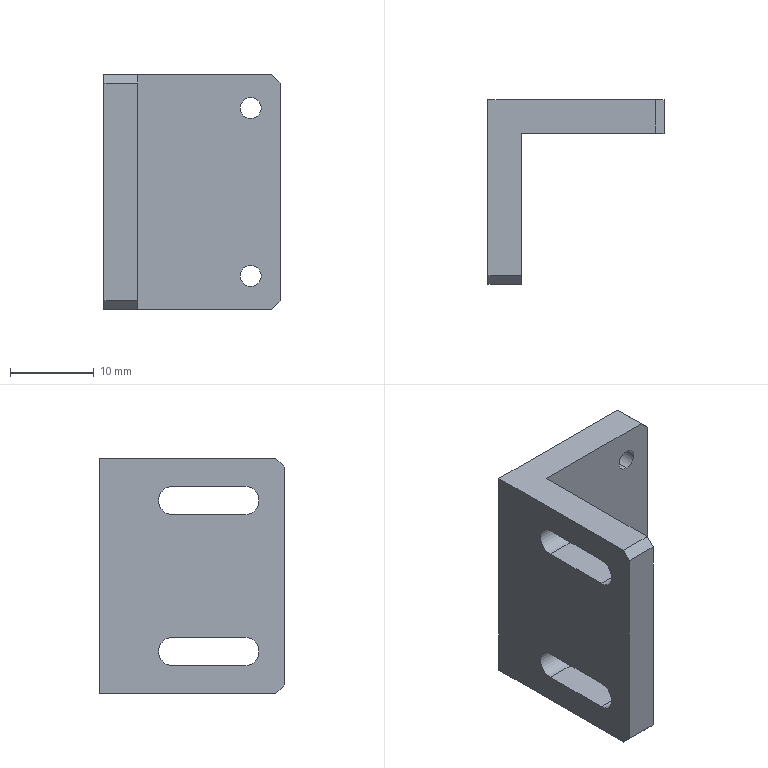Part | NX | features BREP 1 | 1 solid | 24 faces | box 21 x 22 x 28 mm | volume 4014 mm3 | plane 16 | cylinder 8 | commonest cylinder face diameters 2.5 x4 3.4 x4
STEP:
#1=CARTESIAN_POINT('',(16.,18.,-14.));
#2=VERTEX_POINT('',#1);
#3=CARTESIAN_POINT('',(17.,18.,-13.));
#4=VERTEX_POINT('',#3);
#5=CARTESIAN_POINT('',(17.,18.,-13.));
#6=DIRECTION('',(0.7071,0.,0.7071));
#7=VECTOR('',#6,1000.);
#8=LINE('',#5,#7);
#9=EDGE_CURVE('',#2,#4,#8,.T.);
#10=ORIENTED_EDGE('',*,*,#9,.F.);
#11=CARTESIAN_POINT('',(16.,22.,-14.));
#12=VERTEX_POINT('',#11);
#13=CARTESIAN_POINT('',(16.,0.,-14.));
#14=DIRECTION('',(0.,-1.,0.));
#15=VECTOR('',#14,1000.);
#16=LINE('',#13,#15);
#17=EDGE_CURVE('',#12,#2,#16,.T.);
#18=ORIENTED_EDGE('',*,*,#17,.F.);
#19=CARTESIAN_POINT('',(17.,22.,-13.));
#20=VERTEX_POINT('',#19);
#21=CARTESIAN_POINT('',(17.,22.,-13.));
#22=DIRECTION('',(-0.7071,0.,-0.7071));
#23=VECTOR('',#22,1000.);
#24=LINE('',#21,#23);
#25=EDGE_CURVE('',#20,#12,#24,.T.);
#26=ORIENTED_EDGE('',*,*,#25,.F.);
#27=CARTESIAN_POINT('',(17.,18.,-13.));
#28=DIRECTION('',(0.,1.,0.));
#29=VECTOR('',#28,1000.);
#30=LINE('',#27,#29);
#31=EDGE_CURVE('',#4,#20,#30,.T.);
#32=ORIENTED_EDGE('',*,*,#31,.F.);
#33=EDGE_LOOP('',(#10,#18,#26,#32));
#34=FACE_BOUND('',#33,.T.);
#35=CARTESIAN_POINT('',(17.,18.,-13.));
#36=DIRECTION('',(-0.7071,0.,0.7071));
#37=DIRECTION('',(0.,1.,0.));
#38=AXIS2_PLACEMENT_3D('',#35,#36,#37);
#39=PLANE('',#38);
#40=ADVANCED_FACE('',(#34),#39,.F.);
#41=CARTESIAN_POINT('',(-4.,1.,-14.));
#42=VERTEX_POINT('',#41);
#43=CARTESIAN_POINT('',(-4.,0.,-13.));
#44=VERTEX_POINT('',#43);
#45=CARTESIAN_POINT('',(-4.,0.,-13.));
#46=DIRECTION('',(0.,-0.7071,0.7071));
#47=VECTOR('',#46,1000.);
#48=LINE('',#45,#47);
#49=EDGE_CURVE('',#42,#44,#48,.T.);
#50=ORIENTED_EDGE('',*,*,#49,.F.);
#51=CARTESIAN_POINT('',(0.,1.,-14.));
#52=VERTEX_POINT('',#51);
#53=CARTESIAN_POINT('',(0.,1.,-14.));
#54=DIRECTION('',(-1.,0.,0.));
#55=VECTOR('',#54,1000.);
#56=LINE('',#53,#55);
#57=EDGE_CURVE('',#52,#42,#56,.T.);
#58=ORIENTED_EDGE('',*,*,#57,.F.);
#59=CARTESIAN_POINT('',(0.,0.,-13.));
#60=VERTEX_POINT('',#59);
#61=CARTESIAN_POINT('',(0.,0.,-13.));
#62=DIRECTION('',(0.,0.7071,-0.7071));
#63=VECTOR('',#62,1000.);
#64=LINE('',#61,#63);
#65=EDGE_CURVE('',#60,#52,#64,.T.);
#66=ORIENTED_EDGE('',*,*,#65,.F.);
#67=CARTESIAN_POINT('',(-4.,0.,-13.));
#68=DIRECTION('',(1.,0.,0.));
#69=VECTOR('',#68,1000.);
#70=LINE('',#67,#69);
#71=EDGE_CURVE('',#44,#60,#70,.T.);
#72=ORIENTED_EDGE('',*,*,#71,.F.);
#73=EDGE_LOOP('',(#50,#58,#66,#72));
#74=FACE_BOUND('',#73,.T.);
#75=CARTESIAN_POINT('',(-4.,0.,-13.));
#76=DIRECTION('',(0.,0.7071,0.7071));
#77=DIRECTION('',(1.,0.,0.));
#78=AXIS2_PLACEMENT_3D('',#75,#76,#77);
#79=PLANE('',#78);
#80=ADVANCED_FACE('',(#74),#79,.F.);
#81=CARTESIAN_POINT('',(17.,18.,13.));
#82=VERTEX_POINT('',#81);
#83=CARTESIAN_POINT('',(16.,18.,14.));
#84=VERTEX_POINT('',#83);
#85=CARTESIAN_POINT('',(16.,18.,14.));
#86=DIRECTION('',(-0.7071,0.,0.7071));
#87=VECTOR('',#86,1000.);
#88=LINE('',#85,#87);
#89=EDGE_CURVE('',#82,#84,#88,.T.);
#90=ORIENTED_EDGE('',*,*,#89,.F.);
#91=CARTESIAN_POINT('',(17.,22.,13.));
#92=VERTEX_POINT('',#91);
#93=CARTESIAN_POINT('',(17.,18.,13.));
#94=DIRECTION('',(0.,-1.,0.));
#95=VECTOR('',#94,1000.);
#96=LINE('',#93,#95);
#97=EDGE_CURVE('',#92,#82,#96,.T.);
#98=ORIENTED_EDGE('',*,*,#97,.F.);
#99=CARTESIAN_POINT('',(16.,22.,14.));
#100=VERTEX_POINT('',#99);
#101=CARTESIAN_POINT('',(16.,22.,14.));
#102=DIRECTION('',(0.7071,0.,-0.7071));
#103=VECTOR('',#102,1000.);
#104=LINE('',#101,#103);
#105=EDGE_CURVE('',#100,#92,#104,.T.);
#106=ORIENTED_EDGE('',*,*,#105,.F.);
#107=CARTESIAN_POINT('',(16.,22.,14.));
#108=DIRECTION('',(0.,1.,0.));
#109=VECTOR('',#108,1000.);
#110=LINE('',#107,#109);
#111=EDGE_CURVE('',#84,#100,#110,.T.);
#112=ORIENTED_EDGE('',*,*,#111,.F.);
#113=EDGE_LOOP('',(#90,#98,#106,#112));
#114=FACE_BOUND('',#113,.T.);
#115=CARTESIAN_POINT('',(16.,0.,14.));
#116=DIRECTION('',(0.7071,0.,0.7071));
#117=DIRECTION('',(0.,-1.,0.));
#118=AXIS2_PLACEMENT_3D('',#115,#116,#117);
#119=PLANE('',#118);
#120=ADVANCED_FACE('',(#114),#119,.T.);
#121=CARTESIAN_POINT('',(-4.,0.,13.));
#122=VERTEX_POINT('',#121);
#123=CARTESIAN_POINT('',(-4.,1.,14.));
#124=VERTEX_POINT('',#123);
#125=CARTESIAN_POINT('',(-4.,1.,14.));
#126=DIRECTION('',(0.,0.7071,0.7071));
#127=VECTOR('',#126,1000.);
#128=LINE('',#125,#127);
#129=EDGE_CURVE('',#122,#124,#128,.T.);
#130=ORIENTED_EDGE('',*,*,#129,.F.);
#131=CARTESIAN_POINT('',(0.,0.,13.));
#132=VERTEX_POINT('',#131);
#133=CARTESIAN_POINT('',(-4.,0.,13.));
#134=DIRECTION('',(-1.,0.,0.));
#135=VECTOR('',#134,1000.);
#136=LINE('',#133,#135);
#137=EDGE_CURVE('',#132,#122,#136,.T.);
#138=ORIENTED_EDGE('',*,*,#137,.F.);
#139=CARTESIAN_POINT('',(0.,1.,14.));
#140=VERTEX_POINT('',#139);
#141=CARTESIAN_POINT('',(0.,1.,14.));
#142=DIRECTION('',(0.,-0.7071,-0.7071));
#143=VECTOR('',#142,1000.);
#144=LINE('',#141,#143);
#145=EDGE_CURVE('',#140,#132,#144,.T.);
#146=ORIENTED_EDGE('',*,*,#145,.F.);
#147=CARTESIAN_POINT('',(0.,1.,14.));
#148=DIRECTION('',(1.,0.,0.));
#149=VECTOR('',#148,1000.);
#150=LINE('',#147,#149);
#151=EDGE_CURVE('',#124,#140,#150,.T.);
#152=ORIENTED_EDGE('',*,*,#151,.F.);
#153=EDGE_LOOP('',(#130,#138,#146,#152));
#154=FACE_BOUND('',#153,.T.);
#155=CARTESIAN_POINT('',(0.,1.,14.));
#156=DIRECTION('',(0.,-0.7071,0.7071));
#157=DIRECTION('',(-1.,0.,0.));
#158=AXIS2_PLACEMENT_3D('',#155,#156,#157);
#159=PLANE('',#158);
#160=ADVANCED_FACE('',(#154),#159,.T.);
#161=CARTESIAN_POINT('',(0.,13.3,7.3));
#162=VERTEX_POINT('',#161);
#163=CARTESIAN_POINT('',(-4.,13.3,7.3));
#164=VERTEX_POINT('',#163);
#165=CARTESIAN_POINT('',(0.,13.3,7.3));
#166=DIRECTION('',(-1.,0.,0.));
#167=VECTOR('',#166,1000.);
#168=LINE('',#165,#167);
#169=EDGE_CURVE('',#162,#164,#168,.T.);
#170=ORIENTED_EDGE('',*,*,#169,.F.);
#171=CARTESIAN_POINT('',(0.,13.3,10.7));
#172=VERTEX_POINT('',#171);
#173=CARTESIAN_POINT('',(0.,13.3,9.));
#174=DIRECTION('',(1.,0.,0.));
#175=DIRECTION('',(0.,0.,-1.));
#176=AXIS2_PLACEMENT_3D('',#173,#174,#175);
#177=CIRCLE('',#176,1.7);
#178=EDGE_CURVE('',#162,#172,#177,.T.);
#179=ORIENTED_EDGE('',*,*,#178,.T.);
#180=CARTESIAN_POINT('',(-4.,13.3,10.7));
#181=VERTEX_POINT('',#180);
#182=CARTESIAN_POINT('',(0.,13.3,10.7));
#183=DIRECTION('',(1.,0.,0.));
#184=VECTOR('',#183,1000.);
#185=LINE('',#182,#184);
#186=EDGE_CURVE('',#181,#172,#185,.T.);
#187=ORIENTED_EDGE('',*,*,#186,.F.);
#188=CARTESIAN_POINT('',(-4.,13.3,9.));
#189=DIRECTION('',(1.,0.,0.));
#190=DIRECTION('',(0.,0.,-1.));
#191=AXIS2_PLACEMENT_3D('',#188,#189,#190);
#192=CIRCLE('',#191,1.7);
#193=EDGE_CURVE('',#164,#181,#192,.T.);
#194=ORIENTED_EDGE('',*,*,#193,.F.);
#195=EDGE_LOOP('',(#170,#179,#187,#194));
#196=FACE_BOUND('',#195,.T.);
#197=CARTESIAN_POINT('',(0.,13.3,9.));
#198=DIRECTION('',(1.,0.,0.));
#199=DIRECTION('',(0.,0.,-1.));
#200=AXIS2_PLACEMENT_3D('',#197,#198,#199);
#201=CYLINDRICAL_SURFACE('',#200,1.7);
#202=ADVANCED_FACE('',(#196),#201,.F.);
#203=CARTESIAN_POINT('',(0.,4.7,10.7));
#204=VERTEX_POINT('',#203);
#205=CARTESIAN_POINT('',(-4.,4.7,10.7));
#206=VERTEX_POINT('',#205);
#207=CARTESIAN_POINT('',(0.,4.7,10.7));
#208=DIRECTION('',(-1.,0.,0.));
#209=VECTOR('',#208,1000.);
#210=LINE('',#207,#209);
#211=EDGE_CURVE('',#204,#206,#210,.T.);
#212=ORIENTED_EDGE('',*,*,#211,.F.);
#213=CARTESIAN_POINT('',(0.,4.7,7.3));
#214=VERTEX_POINT('',#213);
#215=CARTESIAN_POINT('',(0.,4.7,9.));
#216=DIRECTION('',(1.,0.,0.));
#217=DIRECTION('',(0.,0.,-1.));
#218=AXIS2_PLACEMENT_3D('',#215,#216,#217);
#219=CIRCLE('',#218,1.7);
#220=EDGE_CURVE('',#204,#214,#219,.T.);
#221=ORIENTED_EDGE('',*,*,#220,.T.);
#222=CARTESIAN_POINT('',(-4.,4.7,7.3));
#223=VERTEX_POINT('',#222);
#224=CARTESIAN_POINT('',(0.,4.7,7.3));
#225=DIRECTION('',(1.,0.,0.));
#226=VECTOR('',#225,1000.);
#227=LINE('',#224,#226);
#228=EDGE_CURVE('',#223,#214,#227,.T.);
#229=ORIENTED_EDGE('',*,*,#228,.F.);
#230=CARTESIAN_POINT('',(-4.,4.7,9.));
#231=DIRECTION('',(1.,0.,0.));
#232=DIRECTION('',(0.,0.,-1.));
#233=AXIS2_PLACEMENT_3D('',#230,#231,#232);
#234=CIRCLE('',#233,1.7);
#235=EDGE_CURVE('',#206,#223,#234,.T.);
#236=ORIENTED_EDGE('',*,*,#235,.F.);
#237=EDGE_LOOP('',(#212,#221,#229,#236));
#238=FACE_BOUND('',#237,.T.);
#239=CARTESIAN_POINT('',(0.,4.7,9.));
#240=DIRECTION('',(1.,0.,0.));
#241=DIRECTION('',(0.,0.,-1.));
#242=AXIS2_PLACEMENT_3D('',#239,#240,#241);
#243=CYLINDRICAL_SURFACE('',#242,1.7);
#244=ADVANCED_FACE('',(#238),#243,.F.);
#245=ORIENTED_EDGE('',*,*,#186,.T.);
#246=CARTESIAN_POINT('',(0.,4.7,10.7));
#247=DIRECTION('',(0.,1.,0.));
#248=VECTOR('',#247,1000.);
#249=LINE('',#246,#248);
#250=EDGE_CURVE('',#204,#172,#249,.T.);
#251=ORIENTED_EDGE('',*,*,#250,.F.);
#252=ORIENTED_EDGE('',*,*,#211,.T.);
#253=CARTESIAN_POINT('',(-4.,22.,10.7));
#254=DIRECTION('',(0.,-1.,0.));
#255=VECTOR('',#254,1000.);
#256=LINE('',#253,#255);
#257=EDGE_CURVE('',#181,#206,#256,.T.);
#258=ORIENTED_EDGE('',*,*,#257,.F.);
#259=EDGE_LOOP('',(#245,#251,#252,#258));
#260=FACE_BOUND('',#259,.T.);
#261=CARTESIAN_POINT('',(0.,4.7,10.7));
#262=DIRECTION('',(0.,0.,1.));
#263=DIRECTION('',(1.,0.,0.));
#264=AXIS2_PLACEMENT_3D('',#261,#262,#263);
#265=PLANE('',#264);
#266=ADVANCED_FACE('',(#260),#265,.F.);
#267=ORIENTED_EDGE('',*,*,#228,.T.);
#268=CARTESIAN_POINT('',(0.,4.7,7.3));
#269=DIRECTION('',(0.,1.,0.));
#270=VECTOR('',#269,1000.);
#271=LINE('',#268,#270);
#272=EDGE_CURVE('',#214,#162,#271,.T.);
#273=ORIENTED_EDGE('',*,*,#272,.T.);
#274=ORIENTED_EDGE('',*,*,#169,.T.);
#275=CARTESIAN_POINT('',(-4.,22.,7.3));
#276=DIRECTION('',(0.,1.,0.));
#277=VECTOR('',#276,1000.);
#278=LINE('',#275,#277);
#279=EDGE_CURVE('',#223,#164,#278,.T.);
#280=ORIENTED_EDGE('',*,*,#279,.F.);
#281=EDGE_LOOP('',(#267,#273,#274,#280));
#282=FACE_BOUND('',#281,.T.);
#283=CARTESIAN_POINT('',(0.,4.7,7.3));
#284=DIRECTION('',(0.,0.,-1.));
#285=DIRECTION('',(-1.,0.,0.));
#286=AXIS2_PLACEMENT_3D('',#283,#284,#285);
#287=PLANE('',#286);
#288=ADVANCED_FACE('',(#282),#287,.F.);
#289=CARTESIAN_POINT('',(-4.,13.3,-7.3));
#290=VERTEX_POINT('',#289);
#291=CARTESIAN_POINT('',(0.,13.3,-7.3));
#292=VERTEX_POINT('',#291);
#293=CARTESIAN_POINT('',(0.,13.3,-7.3));
#294=DIRECTION('',(1.,0.,0.));
#295=VECTOR('',#294,1000.);
#296=LINE('',#293,#295);
#297=EDGE_CURVE('',#290,#292,#296,.T.);
#298=ORIENTED_EDGE('',*,*,#297,.T.);
#299=CARTESIAN_POINT('',(0.,4.7,-7.3));
#300=VERTEX_POINT('',#299);
#301=CARTESIAN_POINT('',(0.,4.7,-7.3));
#302=DIRECTION('',(0.,1.,0.));
#303=VECTOR('',#302,1000.);
#304=LINE('',#301,#303);
#305=EDGE_CURVE('',#300,#292,#304,.T.);
#306=ORIENTED_EDGE('',*,*,#305,.F.);
#307=CARTESIAN_POINT('',(-4.,4.7,-7.3));
#308=VERTEX_POINT('',#307);
#309=CARTESIAN_POINT('',(0.,4.7,-7.3));
#310=DIRECTION('',(-1.,0.,0.));
#311=VECTOR('',#310,1000.);
#312=LINE('',#309,#311);
#313=EDGE_CURVE('',#300,#308,#312,.T.);
#314=ORIENTED_EDGE('',*,*,#313,.T.);
#315=CARTESIAN_POINT('',(-4.,22.,-7.3));
#316=DIRECTION('',(0.,-1.,0.));
#317=VECTOR('',#316,1000.);
#318=LINE('',#315,#317);
#319=EDGE_CURVE('',#290,#308,#318,.T.);
#320=ORIENTED_EDGE('',*,*,#319,.F.);
#321=EDGE_LOOP('',(#298,#306,#314,#320));
#322=FACE_BOUND('',#321,.T.);
#323=CARTESIAN_POINT('',(0.,4.7,-7.3));
#324=DIRECTION('',(0.,0.,1.));
#325=DIRECTION('',(1.,0.,0.));
#326=AXIS2_PLACEMENT_3D('',#323,#324,#325);
#327=PLANE('',#326);
#328=ADVANCED_FACE('',(#322),#327,.F.);
#329=CARTESIAN_POINT('',(0.,13.3,-10.7));
#330=VERTEX_POINT('',#329);
#331=CARTESIAN_POINT('',(-4.,13.3,-10.7));
#332=VERTEX_POINT('',#331);
#333=CARTESIAN_POINT('',(0.,13.3,-10.7));
#334=DIRECTION('',(-1.,0.,0.));
#335=VECTOR('',#334,1000.);
#336=LINE('',#333,#335);
#337=EDGE_CURVE('',#330,#332,#336,.T.);
#338=ORIENTED_EDGE('',*,*,#337,.F.);
#339=CARTESIAN_POINT('',(0.,13.3,-9.));
#340=DIRECTION('',(1.,0.,0.));
#341=DIRECTION('',(0.,0.,-1.));
#342=AXIS2_PLACEMENT_3D('',#339,#340,#341);
#343=CIRCLE('',#342,1.7);
#344=EDGE_CURVE('',#330,#292,#343,.T.);
#345=ORIENTED_EDGE('',*,*,#344,.T.);
#346=ORIENTED_EDGE('',*,*,#297,.F.);
#347=CARTESIAN_POINT('',(-4.,13.3,-9.));
#348=DIRECTION('',(1.,0.,0.));
#349=DIRECTION('',(0.,0.,-1.));
#350=AXIS2_PLACEMENT_3D('',#347,#348,#349);
#351=CIRCLE('',#350,1.7);
#352=EDGE_CURVE('',#332,#290,#351,.T.);
#353=ORIENTED_EDGE('',*,*,#352,.F.);
#354=EDGE_LOOP('',(#338,#345,#346,#353));
#355=FACE_BOUND('',#354,.T.);
#356=CARTESIAN_POINT('',(0.,13.3,-9.));
#357=DIRECTION('',(1.,0.,0.));
#358=DIRECTION('',(0.,0.,-1.));
#359=AXIS2_PLACEMENT_3D('',#356,#357,#358);
#360=CYLINDRICAL_SURFACE('',#359,1.7);
#361=ADVANCED_FACE('',(#355),#360,.F.);
#362=ORIENTED_EDGE('',*,*,#313,.F.);
#363=CARTESIAN_POINT('',(0.,4.7,-10.7));
#364=VERTEX_POINT('',#363);
#365=CARTESIAN_POINT('',(0.,4.7,-9.));
#366=DIRECTION('',(1.,0.,0.));
#367=DIRECTION('',(0.,0.,-1.));
#368=AXIS2_PLACEMENT_3D('',#365,#366,#367);
#369=CIRCLE('',#368,1.7);
#370=EDGE_CURVE('',#300,#364,#369,.T.);
#371=ORIENTED_EDGE('',*,*,#370,.T.);
#372=CARTESIAN_POINT('',(-4.,4.7,-10.7));
#373=VERTEX_POINT('',#372);
#374=CARTESIAN_POINT('',(0.,4.7,-10.7));
#375=DIRECTION('',(1.,0.,0.));
#376=VECTOR('',#375,1000.);
#377=LINE('',#374,#376);
#378=EDGE_CURVE('',#373,#364,#377,.T.);
#379=ORIENTED_EDGE('',*,*,#378,.F.);
#380=CARTESIAN_POINT('',(-4.,4.7,-9.));
#381=DIRECTION('',(1.,0.,0.));
#382=DIRECTION('',(0.,0.,-1.));
#383=AXIS2_PLACEMENT_3D('',#380,#381,#382);
#384=CIRCLE('',#383,1.7);
#385=EDGE_CURVE('',#308,#373,#384,.T.);
#386=ORIENTED_EDGE('',*,*,#385,.F.);
#387=EDGE_LOOP('',(#362,#371,#379,#386));
#388=FACE_BOUND('',#387,.T.);
#389=CARTESIAN_POINT('',(0.,4.7,-9.));
#390=DIRECTION('',(1.,0.,0.));
#391=DIRECTION('',(0.,0.,-1.));
#392=AXIS2_PLACEMENT_3D('',#389,#390,#391);
#393=CYLINDRICAL_SURFACE('',#392,1.7);
#394=ADVANCED_FACE('',(#388),#393,.F.);
#395=ORIENTED_EDGE('',*,*,#378,.T.);
#396=CARTESIAN_POINT('',(0.,4.7,-10.7));
#397=DIRECTION('',(0.,1.,0.));
#398=VECTOR('',#397,1000.);
#399=LINE('',#396,#398);
#400=EDGE_CURVE('',#364,#330,#399,.T.);
#401=ORIENTED_EDGE('',*,*,#400,.T.);
#402=ORIENTED_EDGE('',*,*,#337,.T.);
#403=CARTESIAN_POINT('',(-4.,22.,-10.7));
#404=DIRECTION('',(0.,1.,0.));
#405=VECTOR('',#404,1000.);
#406=LINE('',#403,#405);
#407=EDGE_CURVE('',#373,#332,#406,.T.);
#408=ORIENTED_EDGE('',*,*,#407,.F.);
#409=EDGE_LOOP('',(#395,#401,#402,#408));
#410=FACE_BOUND('',#409,.T.);
#411=CARTESIAN_POINT('',(0.,4.7,-10.7));
#412=DIRECTION('',(0.,0.,-1.));
#413=DIRECTION('',(-1.,0.,0.));
#414=AXIS2_PLACEMENT_3D('',#411,#412,#413);
#415=PLANE('',#414);
#416=ADVANCED_FACE('',(#410),#415,.F.);
#417=CARTESIAN_POINT('',(13.5,22.,8.75));
#418=VERTEX_POINT('',#417);
#419=CARTESIAN_POINT('',(13.5,18.,8.75));
#420=VERTEX_POINT('',#419);
#421=CARTESIAN_POINT('',(13.5,22.,8.75));
#422=DIRECTION('',(0.,1.,0.));
#423=VECTOR('',#422,1000.);
#424=LINE('',#421,#423);
#425=EDGE_CURVE('',#418,#420,#424,.F.);
#426=ORIENTED_EDGE('',*,*,#425,.T.);
#427=CARTESIAN_POINT('',(13.5,18.,11.25));
#428=VERTEX_POINT('',#427);
#429=CARTESIAN_POINT('',(13.5,18.,10.));
#430=DIRECTION('',(0.,1.,0.));
#431=DIRECTION('',(0.,0.,1.));
#432=AXIS2_PLACEMENT_3D('',#429,#430,#431);
#433=CIRCLE('',#432,1.25);
#434=EDGE_CURVE('',#428,#420,#433,.T.);
#435=ORIENTED_EDGE('',*,*,#434,.F.);
#436=CARTESIAN_POINT('',(13.5,22.,11.25));
#437=VERTEX_POINT('',#436);
#438=CARTESIAN_POINT('',(13.5,22.,11.25));
#439=DIRECTION('',(0.,1.,0.));
#440=VECTOR('',#439,1000.);
#441=LINE('',#438,#440);
#442=EDGE_CURVE('',#437,#428,#441,.F.);
#443=ORIENTED_EDGE('',*,*,#442,.F.);
#444=CARTESIAN_POINT('',(13.5,22.,10.));
#445=DIRECTION('',(0.,1.,0.));
#446=DIRECTION('',(0.,0.,1.));
#447=AXIS2_PLACEMENT_3D('',#444,#445,#446);
#448=CIRCLE('',#447,1.25);
#449=EDGE_CURVE('',#437,#418,#448,.T.);
#450=ORIENTED_EDGE('',*,*,#449,.T.);
#451=EDGE_LOOP('',(#426,#435,#443,#450));
#452=FACE_BOUND('',#451,.T.);
#453=CARTESIAN_POINT('',(13.5,22.,10.));
#454=DIRECTION('',(0.,1.,0.));
#455=DIRECTION('',(0.,0.,1.));
#456=AXIS2_PLACEMENT_3D('',#453,#454,#455);
#457=CYLINDRICAL_SURFACE('',#456,1.25);
#458=ADVANCED_FACE('',(#452),#457,.F.);
#459=CARTESIAN_POINT('',(13.5,22.,-11.25));
#460=VERTEX_POINT('',#459);
#461=CARTESIAN_POINT('',(13.5,18.,-11.25));
#462=VERTEX_POINT('',#461);
#463=CARTESIAN_POINT('',(13.5,22.,-11.25));
#464=DIRECTION('',(0.,1.,0.));
#465=VECTOR('',#464,1000.);
#466=LINE('',#463,#465);
#467=EDGE_CURVE('',#460,#462,#466,.F.);
#468=ORIENTED_EDGE('',*,*,#467,.T.);
#469=CARTESIAN_POINT('',(13.5,18.,-8.75));
#470=VERTEX_POINT('',#469);
#471=CARTESIAN_POINT('',(13.5,18.,-10.));
#472=DIRECTION('',(0.,1.,0.));
#473=DIRECTION('',(0.,0.,1.));
#474=AXIS2_PLACEMENT_3D('',#471,#472,#473);
#475=CIRCLE('',#474,1.25);
#476=EDGE_CURVE('',#470,#462,#475,.T.);
#477=ORIENTED_EDGE('',*,*,#476,.F.);
#478=CARTESIAN_POINT('',(13.5,22.,-8.75));
#479=VERTEX_POINT('',#478);
#480=CARTESIAN_POINT('',(13.5,22.,-8.75));
#481=DIRECTION('',(0.,1.,0.));
#482=VECTOR('',#481,1000.);
#483=LINE('',#480,#482);
#484=EDGE_CURVE('',#479,#470,#483,.F.);
#485=ORIENTED_EDGE('',*,*,#484,.F.);
#486=CARTESIAN_POINT('',(13.5,22.,-10.));
#487=DIRECTION('',(0.,1.,0.));
#488=DIRECTION('',(0.,0.,1.));
#489=AXIS2_PLACEMENT_3D('',#486,#487,#488);
#490=CIRCLE('',#489,1.25);
#491=EDGE_CURVE('',#479,#460,#490,.T.);
#492=ORIENTED_EDGE('',*,*,#491,.T.);
#493=EDGE_LOOP('',(#468,#477,#485,#492));
#494=FACE_BOUND('',#493,.T.);
#495=CARTESIAN_POINT('',(13.5,22.,-10.));
#496=DIRECTION('',(0.,1.,0.));
#497=DIRECTION('',(0.,0.,1.));
#498=AXIS2_PLACEMENT_3D('',#495,#496,#497);
#499=CYLINDRICAL_SURFACE('',#498,1.25);
#500=ADVANCED_FACE('',(#494),#499,.F.);
#501=CARTESIAN_POINT('',(0.,18.,-14.));
#502=VERTEX_POINT('',#501);
#503=CARTESIAN_POINT('',(0.,0.,-14.));
#504=DIRECTION('',(0.,1.,0.));
#505=VECTOR('',#504,1000.);
#506=LINE('',#503,#505);
#507=EDGE_CURVE('',#52,#502,#506,.T.);
#508=ORIENTED_EDGE('',*,*,#507,.F.);
#509=ORIENTED_EDGE('',*,*,#57,.T.);
#510=CARTESIAN_POINT('',(-4.,22.,-14.));
#511=VERTEX_POINT('',#510);
#512=CARTESIAN_POINT('',(-4.,22.,-14.));
#513=DIRECTION('',(0.,-1.,0.));
#514=VECTOR('',#513,1000.);
#515=LINE('',#512,#514);
#516=EDGE_CURVE('',#511,#42,#515,.T.);
#517=ORIENTED_EDGE('',*,*,#516,.F.);
#518=CARTESIAN_POINT('',(17.,22.,-14.));
#519=DIRECTION('',(-1.,0.,0.));
#520=VECTOR('',#519,1000.);
#521=LINE('',#518,#520);
#522=EDGE_CURVE('',#12,#511,#521,.T.);
#523=ORIENTED_EDGE('',*,*,#522,.F.);
#524=ORIENTED_EDGE('',*,*,#17,.T.);
#525=CARTESIAN_POINT('',(0.,18.,-14.));
#526=DIRECTION('',(1.,0.,0.));
#527=VECTOR('',#526,1000.);
#528=LINE('',#525,#527);
#529=EDGE_CURVE('',#502,#2,#528,.T.);
#530=ORIENTED_EDGE('',*,*,#529,.F.);
#531=EDGE_LOOP('',(#508,#509,#517,#523,#524,#530));
#532=FACE_BOUND('',#531,.T.);
#533=CARTESIAN_POINT('',(0.,0.,-14.));
#534=DIRECTION('',(0.,0.,1.));
#535=DIRECTION('',(1.,0.,0.));
#536=AXIS2_PLACEMENT_3D('',#533,#534,#535);
#537=PLANE('',#536);
#538=ADVANCED_FACE('',(#532),#537,.F.);
#539=CARTESIAN_POINT('',(-4.,22.,14.));
#540=VERTEX_POINT('',#539);
#541=CARTESIAN_POINT('',(-4.,22.,14.));
#542=DIRECTION('',(0.,-1.,0.));
#543=VECTOR('',#542,1000.);
#544=LINE('',#541,#543);
#545=EDGE_CURVE('',#540,#124,#544,.T.);
#546=ORIENTED_EDGE('',*,*,#545,.T.);
#547=ORIENTED_EDGE('',*,*,#151,.T.);
#548=CARTESIAN_POINT('',(0.,18.,14.));
#549=VERTEX_POINT('',#548);
#550=CARTESIAN_POINT('',(0.,0.,14.));
#551=DIRECTION('',(0.,1.,0.));
#552=VECTOR('',#551,1000.);
#553=LINE('',#550,#552);
#554=EDGE_CURVE('',#140,#549,#553,.T.);
#555=ORIENTED_EDGE('',*,*,#554,.T.);
#556=CARTESIAN_POINT('',(0.,18.,14.));
#557=DIRECTION('',(1.,0.,0.));
#558=VECTOR('',#557,1000.);
#559=LINE('',#556,#558);
#560=EDGE_CURVE('',#549,#84,#559,.T.);
#561=ORIENTED_EDGE('',*,*,#560,.T.);
#562=ORIENTED_EDGE('',*,*,#111,.T.);
#563=CARTESIAN_POINT('',(17.,22.,14.));
#564=DIRECTION('',(-1.,0.,0.));
#565=VECTOR('',#564,1000.);
#566=LINE('',#563,#565);
#567=EDGE_CURVE('',#100,#540,#566,.T.);
#568=ORIENTED_EDGE('',*,*,#567,.T.);
#569=EDGE_LOOP('',(#546,#547,#555,#561,#562,#568));
#570=FACE_BOUND('',#569,.T.);
#571=CARTESIAN_POINT('',(0.,0.,14.));
#572=DIRECTION('',(0.,0.,1.));
#573=DIRECTION('',(1.,0.,0.));
#574=AXIS2_PLACEMENT_3D('',#571,#572,#573);
#575=PLANE('',#574);
#576=ADVANCED_FACE('',(#570),#575,.T.);
#577=CARTESIAN_POINT('',(-4.,0.,14.));
#578=DIRECTION('',(0.,0.,-1.));
#579=VECTOR('',#578,1000.);
#580=LINE('',#577,#579);
#581=EDGE_CURVE('',#122,#44,#580,.T.);
#582=ORIENTED_EDGE('',*,*,#581,.F.);
#583=ORIENTED_EDGE('',*,*,#129,.T.);
#584=ORIENTED_EDGE('',*,*,#545,.F.);
#585=CARTESIAN_POINT('',(-4.,22.,14.));
#586=DIRECTION('',(0.,0.,-1.));
#587=VECTOR('',#586,1000.);
#588=LINE('',#585,#587);
#589=EDGE_CURVE('',#540,#511,#588,.T.);
#590=ORIENTED_EDGE('',*,*,#589,.T.);
#591=ORIENTED_EDGE('',*,*,#516,.T.);
#592=ORIENTED_EDGE('',*,*,#49,.T.);
#593=EDGE_LOOP('',(#582,#583,#584,#590,#591,#592));
#594=FACE_BOUND('',#593,.T.);
#595=ORIENTED_EDGE('',*,*,#319,.T.);
#596=ORIENTED_EDGE('',*,*,#385,.T.);
#597=ORIENTED_EDGE('',*,*,#407,.T.);
#598=ORIENTED_EDGE('',*,*,#352,.T.);
#599=EDGE_LOOP('',(#595,#596,#597,#598));
#600=FACE_BOUND('',#599,.T.);
#601=ORIENTED_EDGE('',*,*,#257,.T.);
#602=ORIENTED_EDGE('',*,*,#235,.T.);
#603=ORIENTED_EDGE('',*,*,#279,.T.);
#604=ORIENTED_EDGE('',*,*,#193,.T.);
#605=EDGE_LOOP('',(#601,#602,#603,#604));
#606=FACE_BOUND('',#605,.T.);
#607=CARTESIAN_POINT('',(-4.,22.,14.));
#608=DIRECTION('',(1.,0.,0.));
#609=DIRECTION('',(0.,0.,-1.));
#610=AXIS2_PLACEMENT_3D('',#607,#608,#609);
#611=PLANE('',#610);
#612=ADVANCED_FACE('',(#594,#600,#606),#611,.F.);
#613=ORIENTED_EDGE('',*,*,#567,.F.);
#614=ORIENTED_EDGE('',*,*,#105,.T.);
#615=CARTESIAN_POINT('',(17.,22.,14.));
#616=DIRECTION('',(0.,0.,-1.));
#617=VECTOR('',#616,1000.);
#618=LINE('',#615,#617);
#619=EDGE_CURVE('',#92,#20,#618,.T.);
#620=ORIENTED_EDGE('',*,*,#619,.T.);
#621=ORIENTED_EDGE('',*,*,#25,.T.);
#622=ORIENTED_EDGE('',*,*,#522,.T.);
#623=ORIENTED_EDGE('',*,*,#589,.F.);
#624=EDGE_LOOP('',(#613,#614,#620,#621,#622,#623));
#625=FACE_BOUND('',#624,.T.);
#626=ORIENTED_EDGE('',*,*,#491,.F.);
#627=CARTESIAN_POINT('',(13.5,22.,-10.));
#628=DIRECTION('',(0.,1.,0.));
#629=DIRECTION('',(0.,0.,1.));
#630=AXIS2_PLACEMENT_3D('',#627,#628,#629);
#631=CIRCLE('',#630,1.25);
#632=EDGE_CURVE('',#460,#479,#631,.T.);
#633=ORIENTED_EDGE('',*,*,#632,.F.);
#634=EDGE_LOOP('',(#626,#633));
#635=FACE_BOUND('',#634,.T.);
#636=ORIENTED_EDGE('',*,*,#449,.F.);
#637=CARTESIAN_POINT('',(13.5,22.,10.));
#638=DIRECTION('',(0.,1.,0.));
#639=DIRECTION('',(0.,0.,1.));
#640=AXIS2_PLACEMENT_3D('',#637,#638,#639);
#641=CIRCLE('',#640,1.25);
#642=EDGE_CURVE('',#418,#437,#641,.T.);
#643=ORIENTED_EDGE('',*,*,#642,.F.);
#644=EDGE_LOOP('',(#636,#643));
#645=FACE_BOUND('',#644,.T.);
#646=CARTESIAN_POINT('',(17.,22.,14.));
#647=DIRECTION('',(0.,-1.,0.));
#648=DIRECTION('',(1.,0.,0.));
#649=AXIS2_PLACEMENT_3D('',#646,#647,#648);
#650=PLANE('',#649);
#651=ADVANCED_FACE('',(#625,#635,#645),#650,.F.);
#652=ORIENTED_EDGE('',*,*,#619,.F.);
#653=ORIENTED_EDGE('',*,*,#97,.T.);
#654=CARTESIAN_POINT('',(17.,18.,14.));
#655=DIRECTION('',(0.,0.,-1.));
#656=VECTOR('',#655,1000.);
#657=LINE('',#654,#656);
#658=EDGE_CURVE('',#82,#4,#657,.T.);
#659=ORIENTED_EDGE('',*,*,#658,.T.);
#660=ORIENTED_EDGE('',*,*,#31,.T.);
#661=EDGE_LOOP('',(#652,#653,#659,#660));
#662=FACE_BOUND('',#661,.T.);
#663=CARTESIAN_POINT('',(17.,18.,14.));
#664=DIRECTION('',(-1.,0.,0.));
#665=DIRECTION('',(0.,0.,1.));
#666=AXIS2_PLACEMENT_3D('',#663,#664,#665);
#667=PLANE('',#666);
#668=ADVANCED_FACE('',(#662),#667,.F.);
#669=ORIENTED_EDGE('',*,*,#658,.F.);
#670=ORIENTED_EDGE('',*,*,#89,.T.);
#671=ORIENTED_EDGE('',*,*,#560,.F.);
#672=CARTESIAN_POINT('',(0.,18.,14.));
#673=DIRECTION('',(0.,0.,-1.));
#674=VECTOR('',#673,1000.);
#675=LINE('',#672,#674);
#676=EDGE_CURVE('',#549,#502,#675,.T.);
#677=ORIENTED_EDGE('',*,*,#676,.T.);
#678=ORIENTED_EDGE('',*,*,#529,.T.);
#679=ORIENTED_EDGE('',*,*,#9,.T.);
#680=EDGE_LOOP('',(#669,#670,#671,#677,#678,#679));
#681=FACE_BOUND('',#680,.T.);
#682=ORIENTED_EDGE('',*,*,#476,.T.);
#683=CARTESIAN_POINT('',(13.5,18.,-10.));
#684=DIRECTION('',(0.,1.,0.));
#685=DIRECTION('',(0.,0.,1.));
#686=AXIS2_PLACEMENT_3D('',#683,#684,#685);
#687=CIRCLE('',#686,1.25);
#688=EDGE_CURVE('',#462,#470,#687,.T.);
#689=ORIENTED_EDGE('',*,*,#688,.T.);
#690=EDGE_LOOP('',(#682,#689));
#691=FACE_BOUND('',#690,.T.);
#692=ORIENTED_EDGE('',*,*,#434,.T.);
#693=CARTESIAN_POINT('',(13.5,18.,10.));
#694=DIRECTION('',(0.,1.,0.));
#695=DIRECTION('',(0.,0.,1.));
#696=AXIS2_PLACEMENT_3D('',#693,#694,#695);
#697=CIRCLE('',#696,1.25);
#698=EDGE_CURVE('',#420,#428,#697,.T.);
#699=ORIENTED_EDGE('',*,*,#698,.T.);
#700=EDGE_LOOP('',(#692,#699));
#701=FACE_BOUND('',#700,.T.);
#702=CARTESIAN_POINT('',(0.,18.,14.));
#703=DIRECTION('',(0.,1.,0.));
#704=DIRECTION('',(0.,0.,1.));
#705=AXIS2_PLACEMENT_3D('',#702,#703,#704);
#706=PLANE('',#705);
#707=ADVANCED_FACE('',(#681,#691,#701),#706,.F.);
#708=CARTESIAN_POINT('',(0.,0.,14.));
#709=DIRECTION('',(0.,0.,-1.));
#710=VECTOR('',#709,1000.);
#711=LINE('',#708,#710);
#712=EDGE_CURVE('',#132,#60,#711,.T.);
#713=ORIENTED_EDGE('',*,*,#712,.F.);
#714=ORIENTED_EDGE('',*,*,#137,.T.);
#715=ORIENTED_EDGE('',*,*,#581,.T.);
#716=ORIENTED_EDGE('',*,*,#71,.T.);
#717=EDGE_LOOP('',(#713,#714,#715,#716));
#718=FACE_BOUND('',#717,.T.);
#719=CARTESIAN_POINT('',(-4.,0.,14.));
#720=DIRECTION('',(0.,1.,0.));
#721=DIRECTION('',(0.,0.,1.));
#722=AXIS2_PLACEMENT_3D('',#719,#720,#721);
#723=PLANE('',#722);
#724=ADVANCED_FACE('',(#718),#723,.F.);
#725=ORIENTED_EDGE('',*,*,#400,.F.);
#726=ORIENTED_EDGE('',*,*,#370,.F.);
#727=ORIENTED_EDGE('',*,*,#305,.T.);
#728=ORIENTED_EDGE('',*,*,#344,.F.);
#729=EDGE_LOOP('',(#725,#726,#727,#728));
#730=FACE_BOUND('',#729,.T.);
#731=ORIENTED_EDGE('',*,*,#554,.F.);
#732=ORIENTED_EDGE('',*,*,#145,.T.);
#733=ORIENTED_EDGE('',*,*,#712,.T.);
#734=ORIENTED_EDGE('',*,*,#65,.T.);
#735=ORIENTED_EDGE('',*,*,#507,.T.);
#736=ORIENTED_EDGE('',*,*,#676,.F.);
#737=EDGE_LOOP('',(#731,#732,#733,#734,#735,#736));
#738=FACE_BOUND('',#737,.T.);
#739=ORIENTED_EDGE('',*,*,#178,.F.);
#740=ORIENTED_EDGE('',*,*,#272,.F.);
#741=ORIENTED_EDGE('',*,*,#220,.F.);
#742=ORIENTED_EDGE('',*,*,#250,.T.);
#743=EDGE_LOOP('',(#739,#740,#741,#742));
#744=FACE_BOUND('',#743,.T.);
#745=CARTESIAN_POINT('',(0.,0.,14.));
#746=DIRECTION('',(-1.,0.,0.));
#747=DIRECTION('',(0.,0.,1.));
#748=AXIS2_PLACEMENT_3D('',#745,#746,#747);
#749=PLANE('',#748);
#750=ADVANCED_FACE('',(#730,#738,#744),#749,.F.);
#751=ORIENTED_EDGE('',*,*,#688,.F.);
#752=ORIENTED_EDGE('',*,*,#467,.F.);
#753=ORIENTED_EDGE('',*,*,#632,.T.);
#754=ORIENTED_EDGE('',*,*,#484,.T.);
#755=EDGE_LOOP('',(#751,#752,#753,#754));
#756=FACE_BOUND('',#755,.T.);
#757=CARTESIAN_POINT('',(13.5,22.,-10.));
#758=DIRECTION('',(0.,1.,0.));
#759=DIRECTION('',(0.,0.,1.));
#760=AXIS2_PLACEMENT_3D('',#757,#758,#759);
#761=CYLINDRICAL_SURFACE('',#760,1.25);
#762=ADVANCED_FACE('',(#756),#761,.F.);
#763=ORIENTED_EDGE('',*,*,#698,.F.);
#764=ORIENTED_EDGE('',*,*,#425,.F.);
#765=ORIENTED_EDGE('',*,*,#642,.T.);
#766=ORIENTED_EDGE('',*,*,#442,.T.);
#767=EDGE_LOOP('',(#763,#764,#765,#766));
#768=FACE_BOUND('',#767,.T.);
#769=CARTESIAN_POINT('',(13.5,22.,10.));
#770=DIRECTION('',(0.,1.,0.));
#771=DIRECTION('',(0.,0.,1.));
#772=AXIS2_PLACEMENT_3D('',#769,#770,#771);
#773=CYLINDRICAL_SURFACE('',#772,1.25);
#774=ADVANCED_FACE('',(#768),#773,.F.);
#775=CLOSED_SHELL('',(#40,#80,#120,#160,#202,#244,#266,#288,#328,#361,#394,#416,#458,#500,#538,#576,#612,#651,#668,#707,#724,#750,#762,#774));
#776=MANIFOLD_SOLID_BREP('',#775);
#777=(LENGTH_UNIT()NAMED_UNIT(*)SI_UNIT(.MILLI.,.METRE.));
#778=UNCERTAINTY_MEASURE_WITH_UNIT(LENGTH_MEASURE(0.00001),#777,'','');
#779=(NAMED_UNIT(*)PLANE_ANGLE_UNIT()SI_UNIT($,.RADIAN.));
#780=(NAMED_UNIT(*)SI_UNIT($,.STERADIAN.)SOLID_ANGLE_UNIT());
#781=(GEOMETRIC_REPRESENTATION_CONTEXT(3)GLOBAL_UNCERTAINTY_ASSIGNED_CONTEXT((#778))GLOBAL_UNIT_ASSIGNED_CONTEXT((#777,#779,#780))REPRESENTATION_CONTEXT('',''));
#782=ADVANCED_BREP_SHAPE_REPRESENTATION('',(#776),#781);